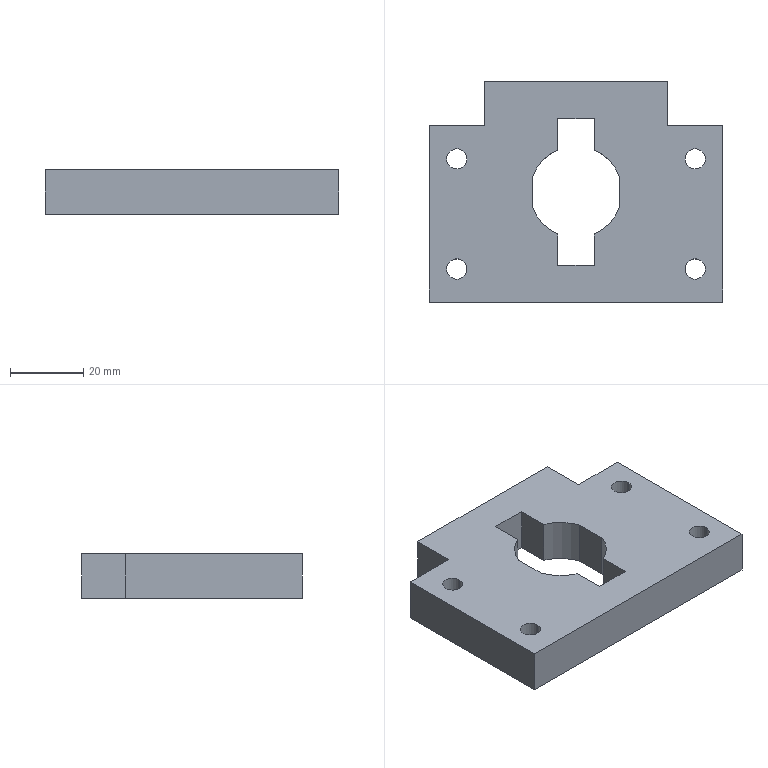Part | STEP file | magnetizing guide plate | 1 solid | 42 faces | box 80 x 60 x 12 mm | volume 43374 mm3 | plane 22 | cylinder 20 | commonest cylinder face diameters 5.5 x8 10 x8 25 x4